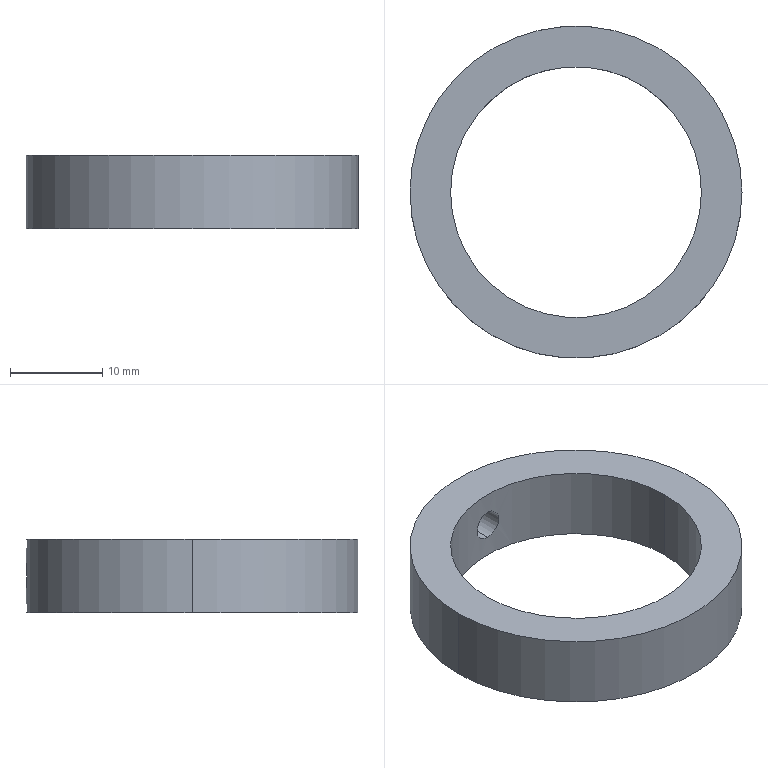Part | SolidWorks | features Extrusion 1, HoleWzd 1 | 1 solid | 8 faces | box 36 x 36 x 8 mm | volume 3457 mm3 | cylinder 6 | plane 2 | commonest cylinder face diameters 3.3 x2 27.2 x2 36 x2
STEP:
#1=CARTESIAN_POINT('',(0.,18.,1.65));
#2=VERTEX_POINT('',#1);
#3=CARTESIAN_POINT('',(0.,18.,-1.65));
#4=VERTEX_POINT('',#3);
#5=CARTESIAN_POINT('',(0.,18.,1.65));
#6=CARTESIAN_POINT('',(-0.2154,18.,1.65));
#7=CARTESIAN_POINT('',(-0.4325,17.996,1.607));
#8=CARTESIAN_POINT('',(-0.8297,17.982,1.442));
#9=CARTESIAN_POINT('',(-1.014,17.972,1.32));
#10=CARTESIAN_POINT('',(-1.242,17.957,1.092));
#11=CARTESIAN_POINT('',(-1.312,17.952,1.007));
#12=CARTESIAN_POINT('',(-1.432,17.943,0.8275));
#13=CARTESIAN_POINT('',(-1.482,17.939,0.7328));
#14=CARTESIAN_POINT('',(-1.565,17.932,0.5332));
#15=CARTESIAN_POINT('',(-1.597,17.929,0.4283));
#16=CARTESIAN_POINT('',(-1.639,17.925,0.2174));
#17=CARTESIAN_POINT('',(-1.65,17.924,0.1103));
#18=CARTESIAN_POINT('',(-1.65,17.924,-0.1077));
#19=CARTESIAN_POINT('',(-1.639,17.925,-0.2151));
#20=CARTESIAN_POINT('',(-1.598,17.929,-0.4261));
#21=CARTESIAN_POINT('',(-1.566,17.932,-0.5308));
#22=CARTESIAN_POINT('',(-1.483,17.939,-0.7307));
#23=CARTESIAN_POINT('',(-1.433,17.943,-0.8255));
#24=CARTESIAN_POINT('',(-1.313,17.952,-1.005));
#25=CARTESIAN_POINT('',(-1.244,17.957,-1.09));
#26=CARTESIAN_POINT('',(-1.015,17.972,-1.318));
#27=CARTESIAN_POINT('',(-0.8317,17.982,-1.441));
#28=CARTESIAN_POINT('',(-0.4348,17.996,-1.606));
#29=CARTESIAN_POINT('',(-0.2181,18.,-1.65));
#30=CARTESIAN_POINT('',(0.,18.,-1.65));
#31=B_SPLINE_CURVE_WITH_KNOTS('',3,(#5,#6,#7,#8,#9,#10,#11,#12,#13,#14,#15,#16,#17,#18,#19,#20,#21,#22,#23,#24,#25,#26,#27,#28,#29,#30),.UNSPECIFIED.,.F.,.F.,(4,2,2,2,2,2,2,2,2,2,2,2,4),(0.005161,0.005806,0.006451,0.006774,0.007096,0.007419,0.007741,0.008064,0.008386,0.008709,0.009031,0.009676,0.01032),.UNSPECIFIED.);
#32=EDGE_CURVE('',#2,#4,#31,.T.);
#33=ORIENTED_EDGE('',*,*,#32,.F.);
#34=CARTESIAN_POINT('',(0.,13.6,1.65));
#35=VERTEX_POINT('',#34);
#36=CARTESIAN_POINT('',(0.,0.,1.65));
#37=DIRECTION('',(0.,-1.,0.));
#38=VECTOR('',#37,1000.);
#39=LINE('',#36,#38);
#40=EDGE_CURVE('',#2,#35,#39,.T.);
#41=ORIENTED_EDGE('',*,*,#40,.T.);
#42=CARTESIAN_POINT('',(0.,13.6,-1.65));
#43=VERTEX_POINT('',#42);
#44=CARTESIAN_POINT('',(0.,13.6,1.65));
#45=CARTESIAN_POINT('',(-0.2154,13.6,1.65));
#46=CARTESIAN_POINT('',(-0.4327,13.595,1.607));
#47=CARTESIAN_POINT('',(-0.8298,13.576,1.442));
#48=CARTESIAN_POINT('',(-1.014,13.563,1.319));
#49=CARTESIAN_POINT('',(-1.242,13.543,1.092));
#50=CARTESIAN_POINT('',(-1.312,13.537,1.007));
#51=CARTESIAN_POINT('',(-1.431,13.525,0.8276));
#52=CARTESIAN_POINT('',(-1.482,13.519,0.733));
#53=CARTESIAN_POINT('',(-1.565,13.51,0.5332));
#54=CARTESIAN_POINT('',(-1.597,13.506,0.4285));
#55=CARTESIAN_POINT('',(-1.639,13.501,0.2175));
#56=CARTESIAN_POINT('',(-1.65,13.5,0.1103));
#57=CARTESIAN_POINT('',(-1.65,13.5,-0.1079));
#58=CARTESIAN_POINT('',(-1.639,13.501,-0.2152));
#59=CARTESIAN_POINT('',(-1.598,13.506,-0.4262));
#60=CARTESIAN_POINT('',(-1.566,13.51,-0.5311));
#61=CARTESIAN_POINT('',(-1.483,13.519,-0.7309));
#62=CARTESIAN_POINT('',(-1.433,13.524,-0.8256));
#63=CARTESIAN_POINT('',(-1.313,13.537,-1.005));
#64=CARTESIAN_POINT('',(-1.243,13.543,-1.09));
#65=CARTESIAN_POINT('',(-1.016,13.563,-1.318));
#66=CARTESIAN_POINT('',(-0.8318,13.576,-1.441));
#67=CARTESIAN_POINT('',(-0.435,13.594,-1.606));
#68=CARTESIAN_POINT('',(-0.2182,13.6,-1.65));
#69=CARTESIAN_POINT('',(0.,13.6,-1.65));
#70=B_SPLINE_CURVE_WITH_KNOTS('',3,(#44,#45,#46,#47,#48,#49,#50,#51,#52,#53,#54,#55,#56,#57,#58,#59,#60,#61,#62,#63,#64,#65,#66,#67,#68,#69),.UNSPECIFIED.,.F.,.F.,(4,2,2,2,2,2,2,2,2,2,2,2,4),(0.005163,0.005809,0.006454,0.006777,0.007099,0.007422,0.007744,0.008067,0.00839,0.008712,0.009035,0.00968,0.01033),.UNSPECIFIED.);
#71=EDGE_CURVE('',#35,#43,#70,.T.);
#72=ORIENTED_EDGE('',*,*,#71,.T.);
#73=CARTESIAN_POINT('',(0.,0.,-1.65));
#74=DIRECTION('',(0.,-1.,0.));
#75=VECTOR('',#74,1000.);
#76=LINE('',#73,#75);
#77=EDGE_CURVE('',#4,#43,#76,.T.);
#78=ORIENTED_EDGE('',*,*,#77,.F.);
#79=EDGE_LOOP('',(#33,#41,#72,#78));
#80=FACE_OUTER_BOUND('',#79,.T.);
#81=CARTESIAN_POINT('',(0.,0.,0.));
#82=DIRECTION('',(0.,-1.,0.));
#83=DIRECTION('',(0.,0.,-1.));
#84=AXIS2_PLACEMENT_3D('',#81,#82,#83);
#85=CYLINDRICAL_SURFACE('',#84,1.65);
#86=ADVANCED_FACE('',(#80),#85,.F.);
#87=CARTESIAN_POINT('',(-13.6,0.,4.));
#88=VERTEX_POINT('',#87);
#89=CARTESIAN_POINT('',(13.6,0.,4.));
#90=VERTEX_POINT('',#89);
#91=CARTESIAN_POINT('',(0.,0.,4.));
#92=DIRECTION('',(0.,0.,1.));
#93=DIRECTION('',(1.,0.,0.));
#94=AXIS2_PLACEMENT_3D('',#91,#92,#93);
#95=CIRCLE('',#94,13.6);
#96=EDGE_CURVE('',#88,#90,#95,.T.);
#97=ORIENTED_EDGE('',*,*,#96,.T.);
#98=CARTESIAN_POINT('',(13.6,0.,-4.));
#99=VERTEX_POINT('',#98);
#100=CARTESIAN_POINT('',(13.6,0.,4.));
#101=DIRECTION('',(0.,0.,-1.));
#102=VECTOR('',#101,1000.);
#103=LINE('',#100,#102);
#104=EDGE_CURVE('',#90,#99,#103,.T.);
#105=ORIENTED_EDGE('',*,*,#104,.T.);
#106=CARTESIAN_POINT('',(-13.6,0.,-4.));
#107=VERTEX_POINT('',#106);
#108=CARTESIAN_POINT('',(0.,0.,-4.));
#109=DIRECTION('',(0.,0.,1.));
#110=DIRECTION('',(1.,0.,0.));
#111=AXIS2_PLACEMENT_3D('',#108,#109,#110);
#112=CIRCLE('',#111,13.6);
#113=EDGE_CURVE('',#107,#99,#112,.T.);
#114=ORIENTED_EDGE('',*,*,#113,.F.);
#115=CARTESIAN_POINT('',(-13.6,0.,4.));
#116=DIRECTION('',(0.,0.,-1.));
#117=VECTOR('',#116,1000.);
#118=LINE('',#115,#117);
#119=EDGE_CURVE('',#88,#107,#118,.T.);
#120=ORIENTED_EDGE('',*,*,#119,.F.);
#121=EDGE_LOOP('',(#97,#105,#114,#120));
#122=FACE_OUTER_BOUND('',#121,.T.);
#123=CARTESIAN_POINT('',(0.,0.,4.));
#124=DIRECTION('',(0.,0.,-1.));
#125=DIRECTION('',(-1.,0.,0.));
#126=AXIS2_PLACEMENT_3D('',#123,#124,#125);
#127=CYLINDRICAL_SURFACE('',#126,13.6);
#128=ADVANCED_FACE('',(#122),#127,.F.);
#129=CARTESIAN_POINT('',(0.,18.,-1.65));
#130=CARTESIAN_POINT('',(0.1091,18.,-1.65));
#131=CARTESIAN_POINT('',(0.2163,17.999,-1.639));
#132=CARTESIAN_POINT('',(0.4273,17.995,-1.597));
#133=CARTESIAN_POINT('',(0.5321,17.992,-1.566));
#134=CARTESIAN_POINT('',(0.7319,17.985,-1.483));
#135=CARTESIAN_POINT('',(0.8267,17.981,-1.432));
#136=CARTESIAN_POINT('',(1.006,17.972,-1.312));
#137=CARTESIAN_POINT('',(1.091,17.967,-1.243));
#138=CARTESIAN_POINT('',(1.319,17.952,-1.014));
#139=CARTESIAN_POINT('',(1.442,17.942,-0.8303));
#140=CARTESIAN_POINT('',(1.607,17.928,-0.4332));
#141=CARTESIAN_POINT('',(1.65,17.924,-0.216));
#142=CARTESIAN_POINT('',(1.65,17.924,0.1071));
#143=CARTESIAN_POINT('',(1.639,17.925,0.2165));
#144=CARTESIAN_POINT('',(1.597,17.929,0.4281));
#145=CARTESIAN_POINT('',(1.566,17.932,0.531));
#146=CARTESIAN_POINT('',(1.483,17.939,0.7309));
#147=CARTESIAN_POINT('',(1.432,17.943,0.8274));
#148=CARTESIAN_POINT('',(1.312,17.952,1.006));
#149=CARTESIAN_POINT('',(1.244,17.957,1.089));
#150=CARTESIAN_POINT('',(1.09,17.967,1.244));
#151=CARTESIAN_POINT('',(1.007,17.972,1.312));
#152=CARTESIAN_POINT('',(0.8279,17.981,1.431));
#153=CARTESIAN_POINT('',(0.7314,17.985,1.483));
#154=CARTESIAN_POINT('',(0.5315,17.992,1.566));
#155=CARTESIAN_POINT('',(0.4287,17.995,1.597));
#156=CARTESIAN_POINT('',(0.2171,17.999,1.639));
#157=CARTESIAN_POINT('',(0.1077,18.,1.65));
#158=CARTESIAN_POINT('',(0.,18.,1.65));
#159=B_SPLINE_CURVE_WITH_KNOTS('',3,(#129,#130,#131,#132,#133,#134,#135,#136,#137,#138,#139,#140,#141,#142,#143,#144,#145,#146,#147,#148,#149,#150,#151,#152,#153,#154,#155,#156,#157,#158),.UNSPECIFIED.,.F.,.F.,(4,2,2,2,2,2,2,2,2,2,2,2,2,2,4),(0.,0.0003226,0.0006452,0.0009678,0.00129,0.001936,0.002581,0.002903,0.003226,0.003548,0.003871,0.004194,0.004516,0.004839,0.005161),.UNSPECIFIED.);
#160=EDGE_CURVE('',#4,#2,#159,.T.);
#161=ORIENTED_EDGE('',*,*,#160,.T.);
#162=ORIENTED_EDGE('',*,*,#32,.T.);
#163=EDGE_LOOP('',(#161,#162));
#164=FACE_BOUND('',#163,.T.);
#165=CARTESIAN_POINT('',(18.,0.,4.));
#166=VERTEX_POINT('',#165);
#167=CARTESIAN_POINT('',(-18.,0.,4.));
#168=VERTEX_POINT('',#167);
#169=CARTESIAN_POINT('',(0.,0.,4.));
#170=DIRECTION('',(0.,0.,1.));
#171=DIRECTION('',(1.,0.,0.));
#172=AXIS2_PLACEMENT_3D('',#169,#170,#171);
#173=CIRCLE('',#172,18.);
#174=EDGE_CURVE('',#166,#168,#173,.T.);
#175=ORIENTED_EDGE('',*,*,#174,.F.);
#176=CARTESIAN_POINT('',(18.,0.,-4.));
#177=VERTEX_POINT('',#176);
#178=CARTESIAN_POINT('',(18.,0.,4.));
#179=DIRECTION('',(0.,0.,-1.));
#180=VECTOR('',#179,1000.);
#181=LINE('',#178,#180);
#182=EDGE_CURVE('',#166,#177,#181,.T.);
#183=ORIENTED_EDGE('',*,*,#182,.T.);
#184=CARTESIAN_POINT('',(-18.,0.,-4.));
#185=VERTEX_POINT('',#184);
#186=CARTESIAN_POINT('',(0.,0.,-4.));
#187=DIRECTION('',(0.,0.,1.));
#188=DIRECTION('',(1.,0.,0.));
#189=AXIS2_PLACEMENT_3D('',#186,#187,#188);
#190=CIRCLE('',#189,18.);
#191=EDGE_CURVE('',#177,#185,#190,.T.);
#192=ORIENTED_EDGE('',*,*,#191,.T.);
#193=CARTESIAN_POINT('',(-18.,0.,4.));
#194=DIRECTION('',(0.,0.,-1.));
#195=VECTOR('',#194,1000.);
#196=LINE('',#193,#195);
#197=EDGE_CURVE('',#168,#185,#196,.T.);
#198=ORIENTED_EDGE('',*,*,#197,.F.);
#199=EDGE_LOOP('',(#175,#183,#192,#198));
#200=FACE_OUTER_BOUND('',#199,.T.);
#201=CARTESIAN_POINT('',(0.,0.,4.));
#202=DIRECTION('',(0.,0.,-1.));
#203=DIRECTION('',(-1.,0.,0.));
#204=AXIS2_PLACEMENT_3D('',#201,#202,#203);
#205=CYLINDRICAL_SURFACE('',#204,18.);
#206=ADVANCED_FACE('',(#164,#200),#205,.T.);
#207=CARTESIAN_POINT('',(0.,0.,4.));
#208=DIRECTION('',(0.,0.,1.));
#209=DIRECTION('',(1.,0.,0.));
#210=AXIS2_PLACEMENT_3D('',#207,#208,#209);
#211=CIRCLE('',#210,18.);
#212=EDGE_CURVE('',#168,#166,#211,.T.);
#213=ORIENTED_EDGE('',*,*,#212,.T.);
#214=ORIENTED_EDGE('',*,*,#174,.T.);
#215=EDGE_LOOP('',(#213,#214));
#216=FACE_OUTER_BOUND('',#215,.T.);
#217=ORIENTED_EDGE('',*,*,#96,.F.);
#218=CARTESIAN_POINT('',(0.,0.,4.));
#219=DIRECTION('',(0.,0.,1.));
#220=DIRECTION('',(1.,0.,0.));
#221=AXIS2_PLACEMENT_3D('',#218,#219,#220);
#222=CIRCLE('',#221,13.6);
#223=EDGE_CURVE('',#90,#88,#222,.T.);
#224=ORIENTED_EDGE('',*,*,#223,.F.);
#225=EDGE_LOOP('',(#217,#224));
#226=FACE_BOUND('',#225,.T.);
#227=CARTESIAN_POINT('',(0.,0.,4.));
#228=DIRECTION('',(0.,0.,1.));
#229=DIRECTION('',(1.,0.,0.));
#230=AXIS2_PLACEMENT_3D('',#227,#228,#229);
#231=PLANE('',#230);
#232=ADVANCED_FACE('',(#216,#226),#231,.T.);
#233=CARTESIAN_POINT('',(0.,0.,-4.));
#234=DIRECTION('',(0.,0.,1.));
#235=DIRECTION('',(1.,0.,0.));
#236=AXIS2_PLACEMENT_3D('',#233,#234,#235);
#237=CIRCLE('',#236,18.);
#238=EDGE_CURVE('',#185,#177,#237,.T.);
#239=ORIENTED_EDGE('',*,*,#238,.F.);
#240=ORIENTED_EDGE('',*,*,#191,.F.);
#241=EDGE_LOOP('',(#239,#240));
#242=FACE_OUTER_BOUND('',#241,.T.);
#243=ORIENTED_EDGE('',*,*,#113,.T.);
#244=CARTESIAN_POINT('',(0.,0.,-4.));
#245=DIRECTION('',(0.,0.,1.));
#246=DIRECTION('',(1.,0.,0.));
#247=AXIS2_PLACEMENT_3D('',#244,#245,#246);
#248=CIRCLE('',#247,13.6);
#249=EDGE_CURVE('',#99,#107,#248,.T.);
#250=ORIENTED_EDGE('',*,*,#249,.T.);
#251=EDGE_LOOP('',(#243,#250));
#252=FACE_BOUND('',#251,.T.);
#253=CARTESIAN_POINT('',(0.,0.,-4.));
#254=DIRECTION('',(0.,0.,1.));
#255=DIRECTION('',(1.,0.,0.));
#256=AXIS2_PLACEMENT_3D('',#253,#254,#255);
#257=PLANE('',#256);
#258=ADVANCED_FACE('',(#242,#252),#257,.F.);
#259=ORIENTED_EDGE('',*,*,#182,.F.);
#260=ORIENTED_EDGE('',*,*,#212,.F.);
#261=ORIENTED_EDGE('',*,*,#197,.T.);
#262=ORIENTED_EDGE('',*,*,#238,.T.);
#263=EDGE_LOOP('',(#259,#260,#261,#262));
#264=FACE_OUTER_BOUND('',#263,.T.);
#265=CARTESIAN_POINT('',(0.,0.,4.));
#266=DIRECTION('',(0.,0.,-1.));
#267=DIRECTION('',(-1.,0.,0.));
#268=AXIS2_PLACEMENT_3D('',#265,#266,#267);
#269=CYLINDRICAL_SURFACE('',#268,18.);
#270=ADVANCED_FACE('',(#264),#269,.T.);
#271=ORIENTED_EDGE('',*,*,#104,.F.);
#272=ORIENTED_EDGE('',*,*,#223,.T.);
#273=ORIENTED_EDGE('',*,*,#119,.T.);
#274=ORIENTED_EDGE('',*,*,#249,.F.);
#275=EDGE_LOOP('',(#271,#272,#273,#274));
#276=FACE_OUTER_BOUND('',#275,.T.);
#277=CARTESIAN_POINT('',(0.,13.6,-1.65));
#278=CARTESIAN_POINT('',(0.1091,13.6,-1.65));
#279=CARTESIAN_POINT('',(0.2164,13.599,-1.639));
#280=CARTESIAN_POINT('',(0.4274,13.594,-1.597));
#281=CARTESIAN_POINT('',(0.5323,13.59,-1.566));
#282=CARTESIAN_POINT('',(0.7321,13.581,-1.483));
#283=CARTESIAN_POINT('',(0.8268,13.575,-1.432));
#284=CARTESIAN_POINT('',(1.006,13.563,-1.312));
#285=CARTESIAN_POINT('',(1.091,13.556,-1.243));
#286=CARTESIAN_POINT('',(1.319,13.537,-1.014));
#287=CARTESIAN_POINT('',(1.442,13.524,-0.8304));
#288=CARTESIAN_POINT('',(1.607,13.505,-0.4334));
#289=CARTESIAN_POINT('',(1.65,13.5,-0.2161));
#290=CARTESIAN_POINT('',(1.65,13.5,0.1071));
#291=CARTESIAN_POINT('',(1.639,13.501,0.2166));
#292=CARTESIAN_POINT('',(1.597,13.506,0.4283));
#293=CARTESIAN_POINT('',(1.566,13.51,0.5312));
#294=CARTESIAN_POINT('',(1.483,13.519,0.7311));
#295=CARTESIAN_POINT('',(1.432,13.525,0.8275));
#296=CARTESIAN_POINT('',(1.312,13.537,1.006));
#297=CARTESIAN_POINT('',(1.244,13.543,1.09));
#298=CARTESIAN_POINT('',(1.09,13.556,1.244));
#299=CARTESIAN_POINT('',(1.007,13.563,1.312));
#300=CARTESIAN_POINT('',(0.828,13.575,1.431));
#301=CARTESIAN_POINT('',(0.7315,13.581,1.483));
#302=CARTESIAN_POINT('',(0.5317,13.59,1.566));
#303=CARTESIAN_POINT('',(0.4288,13.594,1.597));
#304=CARTESIAN_POINT('',(0.2172,13.599,1.639));
#305=CARTESIAN_POINT('',(0.1077,13.6,1.65));
#306=CARTESIAN_POINT('',(0.,13.6,1.65));
#307=B_SPLINE_CURVE_WITH_KNOTS('',3,(#277,#278,#279,#280,#281,#282,#283,#284,#285,#286,#287,#288,#289,#290,#291,#292,#293,#294,#295,#296,#297,#298,#299,#300,#301,#302,#303,#304,#305,#306),.UNSPECIFIED.,.F.,.F.,(4,2,2,2,2,2,2,2,2,2,2,2,2,2,4),(0.,0.0003227,0.0006454,0.0009681,0.001291,0.001936,0.002582,0.002904,0.003227,0.00355,0.003873,0.004195,0.004518,0.004841,0.005163),.UNSPECIFIED.);
#308=EDGE_CURVE('',#43,#35,#307,.T.);
#309=ORIENTED_EDGE('',*,*,#308,.F.);
#310=ORIENTED_EDGE('',*,*,#71,.F.);
#311=EDGE_LOOP('',(#309,#310));
#312=FACE_BOUND('',#311,.T.);
#313=CARTESIAN_POINT('',(0.,0.,4.));
#314=DIRECTION('',(0.,0.,-1.));
#315=DIRECTION('',(-1.,0.,0.));
#316=AXIS2_PLACEMENT_3D('',#313,#314,#315);
#317=CYLINDRICAL_SURFACE('',#316,13.6);
#318=ADVANCED_FACE('',(#276,#312),#317,.F.);
#319=ORIENTED_EDGE('',*,*,#40,.F.);
#320=ORIENTED_EDGE('',*,*,#160,.F.);
#321=ORIENTED_EDGE('',*,*,#77,.T.);
#322=ORIENTED_EDGE('',*,*,#308,.T.);
#323=EDGE_LOOP('',(#319,#320,#321,#322));
#324=FACE_OUTER_BOUND('',#323,.T.);
#325=CARTESIAN_POINT('',(0.,0.,0.));
#326=DIRECTION('',(0.,-1.,0.));
#327=DIRECTION('',(0.,0.,-1.));
#328=AXIS2_PLACEMENT_3D('',#325,#326,#327);
#329=CYLINDRICAL_SURFACE('',#328,1.65);
#330=ADVANCED_FACE('',(#324),#329,.F.);
#331=CLOSED_SHELL('',(#86,#128,#206,#232,#258,#270,#318,#330));
#332=MANIFOLD_SOLID_BREP('',#331);
#333=CARTESIAN_POINT('',(0.,0.,0.));
#334=DIRECTION('',(0.,0.,1.));
#335=DIRECTION('',(1.,0.,0.));
#336=AXIS2_PLACEMENT_3D('',#333,#334,#335);
#337=(LENGTH_UNIT()NAMED_UNIT(*)SI_UNIT(.MILLI.,.METRE.));
#338=UNCERTAINTY_MEASURE_WITH_UNIT(LENGTH_MEASURE(0.00001),#337,'','');
#339=(NAMED_UNIT(*)PLANE_ANGLE_UNIT()SI_UNIT($,.RADIAN.));
#340=(NAMED_UNIT(*)SI_UNIT($,.STERADIAN.)SOLID_ANGLE_UNIT());
#341=(GEOMETRIC_REPRESENTATION_CONTEXT(3)GLOBAL_UNCERTAINTY_ASSIGNED_CONTEXT((#338))GLOBAL_UNIT_ASSIGNED_CONTEXT((#337,#339,#340))REPRESENTATION_CONTEXT('',''));
#342=ADVANCED_BREP_SHAPE_REPRESENTATION('',(#332,#336),#341);